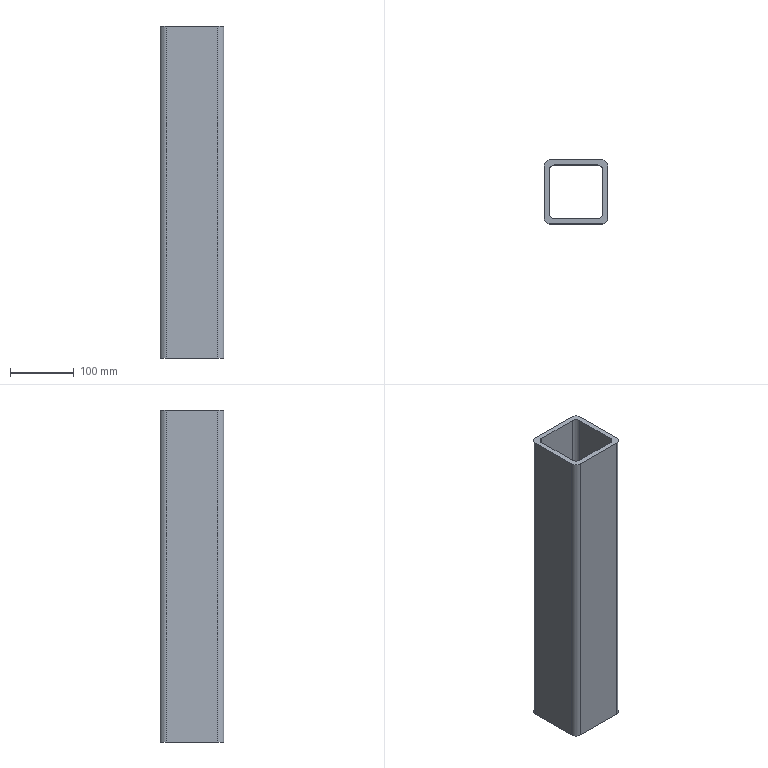Part | SolidWorks | features BaseBody 1 | 1 solid | 18 faces | box 100 x 100 x 520 mm | volume 1514811 mm3 | plane 10 | cylinder 8 | commonest cylinder face diameters 16 x4 20 x4
STEP:
#1=CARTESIAN_POINT('',(90.,-3.65,520.));
#2=VERTEX_POINT('',#1);
#3=CARTESIAN_POINT('',(90.,-3.65,0.));
#4=VERTEX_POINT('',#3);
#5=CARTESIAN_POINT('',(90.,-3.65,520.));
#6=DIRECTION('',(0.,0.,-1.));
#7=VECTOR('',#6,1000.);
#8=LINE('',#5,#7);
#9=EDGE_CURVE('',#2,#4,#8,.T.);
#10=ORIENTED_EDGE('',*,*,#9,.F.);
#11=CARTESIAN_POINT('',(10.,-3.65,520.));
#12=VERTEX_POINT('',#11);
#13=CARTESIAN_POINT('',(10.,-3.65,520.));
#14=DIRECTION('',(1.,0.,0.));
#15=VECTOR('',#14,1000.);
#16=LINE('',#13,#15);
#17=EDGE_CURVE('',#12,#2,#16,.T.);
#18=ORIENTED_EDGE('',*,*,#17,.F.);
#19=CARTESIAN_POINT('',(10.,-3.65,0.));
#20=VERTEX_POINT('',#19);
#21=CARTESIAN_POINT('',(10.,-3.65,520.));
#22=DIRECTION('',(0.,0.,1.));
#23=VECTOR('',#22,1000.);
#24=LINE('',#21,#23);
#25=EDGE_CURVE('',#20,#12,#24,.T.);
#26=ORIENTED_EDGE('',*,*,#25,.F.);
#27=CARTESIAN_POINT('',(10.,-3.65,0.));
#28=DIRECTION('',(-1.,0.,0.));
#29=VECTOR('',#28,1000.);
#30=LINE('',#27,#29);
#31=EDGE_CURVE('',#4,#20,#30,.T.);
#32=ORIENTED_EDGE('',*,*,#31,.F.);
#33=EDGE_LOOP('',(#10,#18,#26,#32));
#34=FACE_OUTER_BOUND('',#33,.T.);
#35=CARTESIAN_POINT('',(10.,-3.65,520.));
#36=DIRECTION('',(0.,1.,0.));
#37=DIRECTION('',(-1.,0.,0.));
#38=AXIS2_PLACEMENT_3D('',#35,#36,#37);
#39=PLANE('',#38);
#40=ADVANCED_FACE('',(#34),#39,.F.);
#41=CARTESIAN_POINT('',(84.,4.35,0.));
#42=VERTEX_POINT('',#41);
#43=CARTESIAN_POINT('',(16.,4.35,0.));
#44=VERTEX_POINT('',#43);
#45=CARTESIAN_POINT('',(10.,4.35,0.));
#46=DIRECTION('',(-1.,0.,0.));
#47=VECTOR('',#46,1000.);
#48=LINE('',#45,#47);
#49=EDGE_CURVE('',#42,#44,#48,.T.);
#50=ORIENTED_EDGE('',*,*,#49,.F.);
#51=CARTESIAN_POINT('',(92.,12.35,0.));
#52=VERTEX_POINT('',#51);
#53=CARTESIAN_POINT('',(84.,12.35,0.));
#54=DIRECTION('',(0.,0.,-1.));
#55=DIRECTION('',(-1.,0.,0.));
#56=AXIS2_PLACEMENT_3D('',#53,#54,#55);
#57=CIRCLE('',#56,8.);
#58=EDGE_CURVE('',#52,#42,#57,.T.);
#59=ORIENTED_EDGE('',*,*,#58,.F.);
#60=CARTESIAN_POINT('',(92.,80.35,0.));
#61=VERTEX_POINT('',#60);
#62=CARTESIAN_POINT('',(92.,6.35,0.));
#63=DIRECTION('',(0.,-1.,0.));
#64=VECTOR('',#63,1000.);
#65=LINE('',#62,#64);
#66=EDGE_CURVE('',#61,#52,#65,.T.);
#67=ORIENTED_EDGE('',*,*,#66,.F.);
#68=CARTESIAN_POINT('',(84.,88.35,0.));
#69=VERTEX_POINT('',#68);
#70=CARTESIAN_POINT('',(84.,80.35,0.));
#71=DIRECTION('',(0.,0.,-1.));
#72=DIRECTION('',(-1.,0.,0.));
#73=AXIS2_PLACEMENT_3D('',#70,#71,#72);
#74=CIRCLE('',#73,8.);
#75=EDGE_CURVE('',#69,#61,#74,.T.);
#76=ORIENTED_EDGE('',*,*,#75,.F.);
#77=CARTESIAN_POINT('',(16.,88.35,0.));
#78=VERTEX_POINT('',#77);
#79=CARTESIAN_POINT('',(10.,88.35,0.));
#80=DIRECTION('',(1.,0.,0.));
#81=VECTOR('',#80,1000.);
#82=LINE('',#79,#81);
#83=EDGE_CURVE('',#78,#69,#82,.T.);
#84=ORIENTED_EDGE('',*,*,#83,.F.);
#85=CARTESIAN_POINT('',(8.,80.35,0.));
#86=VERTEX_POINT('',#85);
#87=CARTESIAN_POINT('',(16.,80.35,0.));
#88=DIRECTION('',(0.,0.,-1.));
#89=DIRECTION('',(-1.,0.,0.));
#90=AXIS2_PLACEMENT_3D('',#87,#88,#89);
#91=CIRCLE('',#90,8.);
#92=EDGE_CURVE('',#86,#78,#91,.T.);
#93=ORIENTED_EDGE('',*,*,#92,.F.);
#94=CARTESIAN_POINT('',(8.,12.35,0.));
#95=VERTEX_POINT('',#94);
#96=CARTESIAN_POINT('',(8.,6.35,0.));
#97=DIRECTION('',(0.,1.,0.));
#98=VECTOR('',#97,1000.);
#99=LINE('',#96,#98);
#100=EDGE_CURVE('',#95,#86,#99,.T.);
#101=ORIENTED_EDGE('',*,*,#100,.F.);
#102=CARTESIAN_POINT('',(16.,12.35,0.));
#103=DIRECTION('',(0.,0.,-1.));
#104=DIRECTION('',(-1.,0.,0.));
#105=AXIS2_PLACEMENT_3D('',#102,#103,#104);
#106=CIRCLE('',#105,8.);
#107=EDGE_CURVE('',#44,#95,#106,.T.);
#108=ORIENTED_EDGE('',*,*,#107,.F.);
#109=EDGE_LOOP('',(#50,#59,#67,#76,#84,#93,#101,#108));
#110=FACE_BOUND('',#109,.T.);
#111=CARTESIAN_POINT('',(0.,86.35,0.));
#112=VERTEX_POINT('',#111);
#113=CARTESIAN_POINT('',(0.,6.35,0.));
#114=VERTEX_POINT('',#113);
#115=CARTESIAN_POINT('',(0.,6.35,0.));
#116=DIRECTION('',(0.,-1.,0.));
#117=VECTOR('',#116,1000.);
#118=LINE('',#115,#117);
#119=EDGE_CURVE('',#112,#114,#118,.T.);
#120=ORIENTED_EDGE('',*,*,#119,.F.);
#121=CARTESIAN_POINT('',(10.,96.35,0.));
#122=VERTEX_POINT('',#121);
#123=CARTESIAN_POINT('',(10.,86.35,0.));
#124=DIRECTION('',(0.,0.,1.));
#125=DIRECTION('',(-1.,0.,0.));
#126=AXIS2_PLACEMENT_3D('',#123,#124,#125);
#127=CIRCLE('',#126,10.);
#128=EDGE_CURVE('',#122,#112,#127,.T.);
#129=ORIENTED_EDGE('',*,*,#128,.F.);
#130=CARTESIAN_POINT('',(90.,96.35,0.));
#131=VERTEX_POINT('',#130);
#132=CARTESIAN_POINT('',(10.,96.35,0.));
#133=DIRECTION('',(-1.,0.,0.));
#134=VECTOR('',#133,1000.);
#135=LINE('',#132,#134);
#136=EDGE_CURVE('',#131,#122,#135,.T.);
#137=ORIENTED_EDGE('',*,*,#136,.F.);
#138=CARTESIAN_POINT('',(100.,86.35,0.));
#139=VERTEX_POINT('',#138);
#140=CARTESIAN_POINT('',(90.,86.35,0.));
#141=DIRECTION('',(0.,0.,1.));
#142=DIRECTION('',(-1.,0.,0.));
#143=AXIS2_PLACEMENT_3D('',#140,#141,#142);
#144=CIRCLE('',#143,10.);
#145=EDGE_CURVE('',#139,#131,#144,.T.);
#146=ORIENTED_EDGE('',*,*,#145,.F.);
#147=CARTESIAN_POINT('',(100.,6.35,0.));
#148=VERTEX_POINT('',#147);
#149=CARTESIAN_POINT('',(100.,6.35,0.));
#150=DIRECTION('',(0.,1.,0.));
#151=VECTOR('',#150,1000.);
#152=LINE('',#149,#151);
#153=EDGE_CURVE('',#148,#139,#152,.T.);
#154=ORIENTED_EDGE('',*,*,#153,.F.);
#155=CARTESIAN_POINT('',(90.,6.35,0.));
#156=DIRECTION('',(0.,0.,1.));
#157=DIRECTION('',(-1.,0.,0.));
#158=AXIS2_PLACEMENT_3D('',#155,#156,#157);
#159=CIRCLE('',#158,10.);
#160=EDGE_CURVE('',#4,#148,#159,.T.);
#161=ORIENTED_EDGE('',*,*,#160,.F.);
#162=ORIENTED_EDGE('',*,*,#31,.T.);
#163=CARTESIAN_POINT('',(10.,6.35,0.));
#164=DIRECTION('',(0.,0.,1.));
#165=DIRECTION('',(-1.,0.,0.));
#166=AXIS2_PLACEMENT_3D('',#163,#164,#165);
#167=CIRCLE('',#166,10.);
#168=EDGE_CURVE('',#114,#20,#167,.T.);
#169=ORIENTED_EDGE('',*,*,#168,.F.);
#170=EDGE_LOOP('',(#120,#129,#137,#146,#154,#161,#162,#169));
#171=FACE_OUTER_BOUND('',#170,.T.);
#172=CARTESIAN_POINT('',(10.,6.35,0.));
#173=DIRECTION('',(0.,0.,1.));
#174=DIRECTION('',(1.,0.,0.));
#175=AXIS2_PLACEMENT_3D('',#172,#173,#174);
#176=PLANE('',#175);
#177=ADVANCED_FACE('',(#110,#171),#176,.F.);
#178=CARTESIAN_POINT('',(100.,6.35,520.));
#179=VERTEX_POINT('',#178);
#180=CARTESIAN_POINT('',(90.,6.35,520.));
#181=DIRECTION('',(0.,0.,-1.));
#182=DIRECTION('',(-1.,0.,0.));
#183=AXIS2_PLACEMENT_3D('',#180,#181,#182);
#184=CIRCLE('',#183,10.);
#185=EDGE_CURVE('',#179,#2,#184,.T.);
#186=ORIENTED_EDGE('',*,*,#185,.T.);
#187=ORIENTED_EDGE('',*,*,#9,.T.);
#188=ORIENTED_EDGE('',*,*,#160,.T.);
#189=CARTESIAN_POINT('',(100.,6.35,520.));
#190=DIRECTION('',(0.,0.,1.));
#191=VECTOR('',#190,1000.);
#192=LINE('',#189,#191);
#193=EDGE_CURVE('',#148,#179,#192,.T.);
#194=ORIENTED_EDGE('',*,*,#193,.T.);
#195=EDGE_LOOP('',(#186,#187,#188,#194));
#196=FACE_OUTER_BOUND('',#195,.T.);
#197=CARTESIAN_POINT('',(90.,6.35,520.));
#198=DIRECTION('',(0.,0.,-1.));
#199=DIRECTION('',(-1.,0.,0.));
#200=AXIS2_PLACEMENT_3D('',#197,#198,#199);
#201=CYLINDRICAL_SURFACE('',#200,10.);
#202=ADVANCED_FACE('',(#196),#201,.T.);
#203=CARTESIAN_POINT('',(92.,80.35,520.));
#204=VERTEX_POINT('',#203);
#205=CARTESIAN_POINT('',(92.,12.35,520.));
#206=VERTEX_POINT('',#205);
#207=CARTESIAN_POINT('',(92.,6.35,520.));
#208=DIRECTION('',(0.,-1.,0.));
#209=VECTOR('',#208,1000.);
#210=LINE('',#207,#209);
#211=EDGE_CURVE('',#204,#206,#210,.T.);
#212=ORIENTED_EDGE('',*,*,#211,.T.);
#213=CARTESIAN_POINT('',(84.,4.35,520.));
#214=VERTEX_POINT('',#213);
#215=CARTESIAN_POINT('',(84.,12.35,520.));
#216=DIRECTION('',(0.,0.,-1.));
#217=DIRECTION('',(-1.,0.,0.));
#218=AXIS2_PLACEMENT_3D('',#215,#216,#217);
#219=CIRCLE('',#218,8.);
#220=EDGE_CURVE('',#206,#214,#219,.T.);
#221=ORIENTED_EDGE('',*,*,#220,.T.);
#222=CARTESIAN_POINT('',(16.,4.35,520.));
#223=VERTEX_POINT('',#222);
#224=CARTESIAN_POINT('',(10.,4.35,520.));
#225=DIRECTION('',(-1.,0.,0.));
#226=VECTOR('',#225,1000.);
#227=LINE('',#224,#226);
#228=EDGE_CURVE('',#214,#223,#227,.T.);
#229=ORIENTED_EDGE('',*,*,#228,.T.);
#230=CARTESIAN_POINT('',(8.,12.35,520.));
#231=VERTEX_POINT('',#230);
#232=CARTESIAN_POINT('',(16.,12.35,520.));
#233=DIRECTION('',(0.,0.,-1.));
#234=DIRECTION('',(-1.,0.,0.));
#235=AXIS2_PLACEMENT_3D('',#232,#233,#234);
#236=CIRCLE('',#235,8.);
#237=EDGE_CURVE('',#223,#231,#236,.T.);
#238=ORIENTED_EDGE('',*,*,#237,.T.);
#239=CARTESIAN_POINT('',(8.,80.35,520.));
#240=VERTEX_POINT('',#239);
#241=CARTESIAN_POINT('',(8.,6.35,520.));
#242=DIRECTION('',(0.,1.,0.));
#243=VECTOR('',#242,1000.);
#244=LINE('',#241,#243);
#245=EDGE_CURVE('',#231,#240,#244,.T.);
#246=ORIENTED_EDGE('',*,*,#245,.T.);
#247=CARTESIAN_POINT('',(16.,88.35,520.));
#248=VERTEX_POINT('',#247);
#249=CARTESIAN_POINT('',(16.,80.35,520.));
#250=DIRECTION('',(0.,0.,-1.));
#251=DIRECTION('',(-1.,0.,0.));
#252=AXIS2_PLACEMENT_3D('',#249,#250,#251);
#253=CIRCLE('',#252,8.);
#254=EDGE_CURVE('',#240,#248,#253,.T.);
#255=ORIENTED_EDGE('',*,*,#254,.T.);
#256=CARTESIAN_POINT('',(84.,88.35,520.));
#257=VERTEX_POINT('',#256);
#258=CARTESIAN_POINT('',(10.,88.35,520.));
#259=DIRECTION('',(1.,0.,0.));
#260=VECTOR('',#259,1000.);
#261=LINE('',#258,#260);
#262=EDGE_CURVE('',#248,#257,#261,.T.);
#263=ORIENTED_EDGE('',*,*,#262,.T.);
#264=CARTESIAN_POINT('',(84.,80.35,520.));
#265=DIRECTION('',(0.,0.,-1.));
#266=DIRECTION('',(-1.,0.,0.));
#267=AXIS2_PLACEMENT_3D('',#264,#265,#266);
#268=CIRCLE('',#267,8.);
#269=EDGE_CURVE('',#257,#204,#268,.T.);
#270=ORIENTED_EDGE('',*,*,#269,.T.);
#271=EDGE_LOOP('',(#212,#221,#229,#238,#246,#255,#263,#270));
#272=FACE_BOUND('',#271,.T.);
#273=CARTESIAN_POINT('',(10.,96.35,520.));
#274=VERTEX_POINT('',#273);
#275=CARTESIAN_POINT('',(0.,86.35,520.));
#276=VERTEX_POINT('',#275);
#277=CARTESIAN_POINT('',(10.,86.35,520.));
#278=DIRECTION('',(0.,0.,1.));
#279=DIRECTION('',(-1.,0.,0.));
#280=AXIS2_PLACEMENT_3D('',#277,#278,#279);
#281=CIRCLE('',#280,10.);
#282=EDGE_CURVE('',#274,#276,#281,.T.);
#283=ORIENTED_EDGE('',*,*,#282,.T.);
#284=CARTESIAN_POINT('',(0.,6.35,520.));
#285=VERTEX_POINT('',#284);
#286=CARTESIAN_POINT('',(0.,6.35,520.));
#287=DIRECTION('',(0.,-1.,0.));
#288=VECTOR('',#287,1000.);
#289=LINE('',#286,#288);
#290=EDGE_CURVE('',#276,#285,#289,.T.);
#291=ORIENTED_EDGE('',*,*,#290,.T.);
#292=CARTESIAN_POINT('',(10.,6.35,520.));
#293=DIRECTION('',(0.,0.,1.));
#294=DIRECTION('',(-1.,0.,0.));
#295=AXIS2_PLACEMENT_3D('',#292,#293,#294);
#296=CIRCLE('',#295,10.);
#297=EDGE_CURVE('',#285,#12,#296,.T.);
#298=ORIENTED_EDGE('',*,*,#297,.T.);
#299=ORIENTED_EDGE('',*,*,#17,.T.);
#300=ORIENTED_EDGE('',*,*,#185,.F.);
#301=CARTESIAN_POINT('',(100.,86.35,520.));
#302=VERTEX_POINT('',#301);
#303=CARTESIAN_POINT('',(100.,6.35,520.));
#304=DIRECTION('',(0.,1.,0.));
#305=VECTOR('',#304,1000.);
#306=LINE('',#303,#305);
#307=EDGE_CURVE('',#179,#302,#306,.T.);
#308=ORIENTED_EDGE('',*,*,#307,.T.);
#309=CARTESIAN_POINT('',(90.,96.35,520.));
#310=VERTEX_POINT('',#309);
#311=CARTESIAN_POINT('',(90.,86.35,520.));
#312=DIRECTION('',(0.,0.,1.));
#313=DIRECTION('',(-1.,0.,0.));
#314=AXIS2_PLACEMENT_3D('',#311,#312,#313);
#315=CIRCLE('',#314,10.);
#316=EDGE_CURVE('',#302,#310,#315,.T.);
#317=ORIENTED_EDGE('',*,*,#316,.T.);
#318=CARTESIAN_POINT('',(10.,96.35,520.));
#319=DIRECTION('',(-1.,0.,0.));
#320=VECTOR('',#319,1000.);
#321=LINE('',#318,#320);
#322=EDGE_CURVE('',#310,#274,#321,.T.);
#323=ORIENTED_EDGE('',*,*,#322,.T.);
#324=EDGE_LOOP('',(#283,#291,#298,#299,#300,#308,#317,#323));
#325=FACE_OUTER_BOUND('',#324,.T.);
#326=CARTESIAN_POINT('',(10.,6.35,520.));
#327=DIRECTION('',(0.,0.,1.));
#328=DIRECTION('',(1.,0.,0.));
#329=AXIS2_PLACEMENT_3D('',#326,#327,#328);
#330=PLANE('',#329);
#331=ADVANCED_FACE('',(#272,#325),#330,.T.);
#332=ORIENTED_EDGE('',*,*,#297,.F.);
#333=CARTESIAN_POINT('',(0.,6.35,520.));
#334=DIRECTION('',(0.,0.,-1.));
#335=VECTOR('',#334,1000.);
#336=LINE('',#333,#335);
#337=EDGE_CURVE('',#285,#114,#336,.T.);
#338=ORIENTED_EDGE('',*,*,#337,.T.);
#339=ORIENTED_EDGE('',*,*,#168,.T.);
#340=ORIENTED_EDGE('',*,*,#25,.T.);
#341=EDGE_LOOP('',(#332,#338,#339,#340));
#342=FACE_OUTER_BOUND('',#341,.T.);
#343=CARTESIAN_POINT('',(10.,6.35,520.));
#344=DIRECTION('',(0.,0.,-1.));
#345=DIRECTION('',(-1.,0.,0.));
#346=AXIS2_PLACEMENT_3D('',#343,#344,#345);
#347=CYLINDRICAL_SURFACE('',#346,10.);
#348=ADVANCED_FACE('',(#342),#347,.T.);
#349=CARTESIAN_POINT('',(8.,12.35,520.));
#350=DIRECTION('',(0.,0.,-1.));
#351=VECTOR('',#350,1000.);
#352=LINE('',#349,#351);
#353=EDGE_CURVE('',#231,#95,#352,.T.);
#354=ORIENTED_EDGE('',*,*,#353,.F.);
#355=ORIENTED_EDGE('',*,*,#237,.F.);
#356=CARTESIAN_POINT('',(16.,4.35,520.));
#357=DIRECTION('',(0.,0.,1.));
#358=VECTOR('',#357,1000.);
#359=LINE('',#356,#358);
#360=EDGE_CURVE('',#44,#223,#359,.T.);
#361=ORIENTED_EDGE('',*,*,#360,.F.);
#362=ORIENTED_EDGE('',*,*,#107,.T.);
#363=EDGE_LOOP('',(#354,#355,#361,#362));
#364=FACE_OUTER_BOUND('',#363,.T.);
#365=CARTESIAN_POINT('',(16.,12.35,520.));
#366=DIRECTION('',(0.,0.,-1.));
#367=DIRECTION('',(-1.,0.,0.));
#368=AXIS2_PLACEMENT_3D('',#365,#366,#367);
#369=CYLINDRICAL_SURFACE('',#368,8.);
#370=ADVANCED_FACE('',(#364),#369,.F.);
#371=ORIENTED_EDGE('',*,*,#228,.F.);
#372=CARTESIAN_POINT('',(84.,4.35,520.));
#373=DIRECTION('',(0.,0.,-1.));
#374=VECTOR('',#373,1000.);
#375=LINE('',#372,#374);
#376=EDGE_CURVE('',#214,#42,#375,.T.);
#377=ORIENTED_EDGE('',*,*,#376,.T.);
#378=ORIENTED_EDGE('',*,*,#49,.T.);
#379=ORIENTED_EDGE('',*,*,#360,.T.);
#380=EDGE_LOOP('',(#371,#377,#378,#379));
#381=FACE_OUTER_BOUND('',#380,.T.);
#382=CARTESIAN_POINT('',(16.,4.35,520.));
#383=DIRECTION('',(0.,1.,0.));
#384=DIRECTION('',(-1.,0.,0.));
#385=AXIS2_PLACEMENT_3D('',#382,#383,#384);
#386=PLANE('',#385);
#387=ADVANCED_FACE('',(#381),#386,.T.);
#388=ORIENTED_EDGE('',*,*,#376,.F.);
#389=ORIENTED_EDGE('',*,*,#220,.F.);
#390=CARTESIAN_POINT('',(92.,12.35,520.));
#391=DIRECTION('',(0.,0.,1.));
#392=VECTOR('',#391,1000.);
#393=LINE('',#390,#392);
#394=EDGE_CURVE('',#52,#206,#393,.T.);
#395=ORIENTED_EDGE('',*,*,#394,.F.);
#396=ORIENTED_EDGE('',*,*,#58,.T.);
#397=EDGE_LOOP('',(#388,#389,#395,#396));
#398=FACE_OUTER_BOUND('',#397,.T.);
#399=CARTESIAN_POINT('',(84.,12.35,520.));
#400=DIRECTION('',(0.,0.,-1.));
#401=DIRECTION('',(-1.,0.,0.));
#402=AXIS2_PLACEMENT_3D('',#399,#400,#401);
#403=CYLINDRICAL_SURFACE('',#402,8.);
#404=ADVANCED_FACE('',(#398),#403,.F.);
#405=ORIENTED_EDGE('',*,*,#394,.T.);
#406=ORIENTED_EDGE('',*,*,#211,.F.);
#407=CARTESIAN_POINT('',(92.,80.35,520.));
#408=DIRECTION('',(0.,0.,1.));
#409=VECTOR('',#408,1000.);
#410=LINE('',#407,#409);
#411=EDGE_CURVE('',#61,#204,#410,.T.);
#412=ORIENTED_EDGE('',*,*,#411,.F.);
#413=ORIENTED_EDGE('',*,*,#66,.T.);
#414=EDGE_LOOP('',(#405,#406,#412,#413));
#415=FACE_OUTER_BOUND('',#414,.T.);
#416=CARTESIAN_POINT('',(92.,80.35,520.));
#417=DIRECTION('',(1.,0.,0.));
#418=DIRECTION('',(0.,1.,0.));
#419=AXIS2_PLACEMENT_3D('',#416,#417,#418);
#420=PLANE('',#419);
#421=ADVANCED_FACE('',(#415),#420,.F.);
#422=ORIENTED_EDGE('',*,*,#411,.T.);
#423=ORIENTED_EDGE('',*,*,#269,.F.);
#424=CARTESIAN_POINT('',(84.,88.35,520.));
#425=DIRECTION('',(0.,0.,1.));
#426=VECTOR('',#425,1000.);
#427=LINE('',#424,#426);
#428=EDGE_CURVE('',#69,#257,#427,.T.);
#429=ORIENTED_EDGE('',*,*,#428,.F.);
#430=ORIENTED_EDGE('',*,*,#75,.T.);
#431=EDGE_LOOP('',(#422,#423,#429,#430));
#432=FACE_OUTER_BOUND('',#431,.T.);
#433=CARTESIAN_POINT('',(84.,80.35,520.));
#434=DIRECTION('',(0.,0.,-1.));
#435=DIRECTION('',(-1.,0.,0.));
#436=AXIS2_PLACEMENT_3D('',#433,#434,#435);
#437=CYLINDRICAL_SURFACE('',#436,8.);
#438=ADVANCED_FACE('',(#432),#437,.F.);
#439=ORIENTED_EDGE('',*,*,#262,.F.);
#440=CARTESIAN_POINT('',(16.,88.35,520.));
#441=DIRECTION('',(0.,0.,-1.));
#442=VECTOR('',#441,1000.);
#443=LINE('',#440,#442);
#444=EDGE_CURVE('',#248,#78,#443,.T.);
#445=ORIENTED_EDGE('',*,*,#444,.T.);
#446=ORIENTED_EDGE('',*,*,#83,.T.);
#447=ORIENTED_EDGE('',*,*,#428,.T.);
#448=EDGE_LOOP('',(#439,#445,#446,#447));
#449=FACE_OUTER_BOUND('',#448,.T.);
#450=CARTESIAN_POINT('',(84.,88.35,520.));
#451=DIRECTION('',(0.,-1.,0.));
#452=DIRECTION('',(1.,0.,0.));
#453=AXIS2_PLACEMENT_3D('',#450,#451,#452);
#454=PLANE('',#453);
#455=ADVANCED_FACE('',(#449),#454,.T.);
#456=ORIENTED_EDGE('',*,*,#444,.F.);
#457=ORIENTED_EDGE('',*,*,#254,.F.);
#458=CARTESIAN_POINT('',(8.,80.35,520.));
#459=DIRECTION('',(0.,0.,1.));
#460=VECTOR('',#459,1000.);
#461=LINE('',#458,#460);
#462=EDGE_CURVE('',#86,#240,#461,.T.);
#463=ORIENTED_EDGE('',*,*,#462,.F.);
#464=ORIENTED_EDGE('',*,*,#92,.T.);
#465=EDGE_LOOP('',(#456,#457,#463,#464));
#466=FACE_OUTER_BOUND('',#465,.T.);
#467=CARTESIAN_POINT('',(16.,80.35,520.));
#468=DIRECTION('',(0.,0.,-1.));
#469=DIRECTION('',(-1.,0.,0.));
#470=AXIS2_PLACEMENT_3D('',#467,#468,#469);
#471=CYLINDRICAL_SURFACE('',#470,8.);
#472=ADVANCED_FACE('',(#466),#471,.F.);
#473=ORIENTED_EDGE('',*,*,#462,.T.);
#474=ORIENTED_EDGE('',*,*,#245,.F.);
#475=ORIENTED_EDGE('',*,*,#353,.T.);
#476=ORIENTED_EDGE('',*,*,#100,.T.);
#477=EDGE_LOOP('',(#473,#474,#475,#476));
#478=FACE_OUTER_BOUND('',#477,.T.);
#479=CARTESIAN_POINT('',(8.,12.35,520.));
#480=DIRECTION('',(-1.,0.,0.));
#481=DIRECTION('',(0.,-1.,0.));
#482=AXIS2_PLACEMENT_3D('',#479,#480,#481);
#483=PLANE('',#482);
#484=ADVANCED_FACE('',(#478),#483,.F.);
#485=ORIENTED_EDGE('',*,*,#290,.F.);
#486=CARTESIAN_POINT('',(0.,86.35,520.));
#487=DIRECTION('',(0.,0.,-1.));
#488=VECTOR('',#487,1000.);
#489=LINE('',#486,#488);
#490=EDGE_CURVE('',#276,#112,#489,.T.);
#491=ORIENTED_EDGE('',*,*,#490,.T.);
#492=ORIENTED_EDGE('',*,*,#119,.T.);
#493=ORIENTED_EDGE('',*,*,#337,.F.);
#494=EDGE_LOOP('',(#485,#491,#492,#493));
#495=FACE_OUTER_BOUND('',#494,.T.);
#496=CARTESIAN_POINT('',(0.,6.35,520.));
#497=DIRECTION('',(-1.,0.,0.));
#498=DIRECTION('',(0.,-1.,0.));
#499=AXIS2_PLACEMENT_3D('',#496,#497,#498);
#500=PLANE('',#499);
#501=ADVANCED_FACE('',(#495),#500,.T.);
#502=ORIENTED_EDGE('',*,*,#282,.F.);
#503=CARTESIAN_POINT('',(10.,96.35,520.));
#504=DIRECTION('',(0.,0.,-1.));
#505=VECTOR('',#504,1000.);
#506=LINE('',#503,#505);
#507=EDGE_CURVE('',#274,#122,#506,.T.);
#508=ORIENTED_EDGE('',*,*,#507,.T.);
#509=ORIENTED_EDGE('',*,*,#128,.T.);
#510=ORIENTED_EDGE('',*,*,#490,.F.);
#511=EDGE_LOOP('',(#502,#508,#509,#510));
#512=FACE_OUTER_BOUND('',#511,.T.);
#513=CARTESIAN_POINT('',(10.,86.35,520.));
#514=DIRECTION('',(0.,0.,-1.));
#515=DIRECTION('',(-1.,0.,0.));
#516=AXIS2_PLACEMENT_3D('',#513,#514,#515);
#517=CYLINDRICAL_SURFACE('',#516,10.);
#518=ADVANCED_FACE('',(#512),#517,.T.);
#519=ORIENTED_EDGE('',*,*,#507,.F.);
#520=ORIENTED_EDGE('',*,*,#322,.F.);
#521=CARTESIAN_POINT('',(90.,96.35,520.));
#522=DIRECTION('',(0.,0.,1.));
#523=VECTOR('',#522,1000.);
#524=LINE('',#521,#523);
#525=EDGE_CURVE('',#131,#310,#524,.T.);
#526=ORIENTED_EDGE('',*,*,#525,.F.);
#527=ORIENTED_EDGE('',*,*,#136,.T.);
#528=EDGE_LOOP('',(#519,#520,#526,#527));
#529=FACE_OUTER_BOUND('',#528,.T.);
#530=CARTESIAN_POINT('',(90.,96.35,520.));
#531=DIRECTION('',(0.,-1.,0.));
#532=DIRECTION('',(1.,0.,0.));
#533=AXIS2_PLACEMENT_3D('',#530,#531,#532);
#534=PLANE('',#533);
#535=ADVANCED_FACE('',(#529),#534,.F.);
#536=ORIENTED_EDGE('',*,*,#316,.F.);
#537=CARTESIAN_POINT('',(100.,86.35,520.));
#538=DIRECTION('',(0.,0.,-1.));
#539=VECTOR('',#538,1000.);
#540=LINE('',#537,#539);
#541=EDGE_CURVE('',#302,#139,#540,.T.);
#542=ORIENTED_EDGE('',*,*,#541,.T.);
#543=ORIENTED_EDGE('',*,*,#145,.T.);
#544=ORIENTED_EDGE('',*,*,#525,.T.);
#545=EDGE_LOOP('',(#536,#542,#543,#544));
#546=FACE_OUTER_BOUND('',#545,.T.);
#547=CARTESIAN_POINT('',(90.,86.35,520.));
#548=DIRECTION('',(0.,0.,-1.));
#549=DIRECTION('',(-1.,0.,0.));
#550=AXIS2_PLACEMENT_3D('',#547,#548,#549);
#551=CYLINDRICAL_SURFACE('',#550,10.);
#552=ADVANCED_FACE('',(#546),#551,.T.);
#553=ORIENTED_EDGE('',*,*,#307,.F.);
#554=ORIENTED_EDGE('',*,*,#193,.F.);
#555=ORIENTED_EDGE('',*,*,#153,.T.);
#556=ORIENTED_EDGE('',*,*,#541,.F.);
#557=EDGE_LOOP('',(#553,#554,#555,#556));
#558=FACE_OUTER_BOUND('',#557,.T.);
#559=CARTESIAN_POINT('',(100.,86.35,520.));
#560=DIRECTION('',(1.,0.,0.));
#561=DIRECTION('',(0.,0.,-1.));
#562=AXIS2_PLACEMENT_3D('',#559,#560,#561);
#563=PLANE('',#562);
#564=ADVANCED_FACE('',(#558),#563,.T.);
#565=CLOSED_SHELL('',(#40,#177,#202,#331,#348,#370,#387,#404,#421,#438,#455,#472,#484,#501,#518,#535,#552,#564));
#566=MANIFOLD_SOLID_BREP('',#565);
#567=CARTESIAN_POINT('',(0.,0.,0.));
#568=DIRECTION('',(0.,0.,1.));
#569=DIRECTION('',(1.,0.,0.));
#570=AXIS2_PLACEMENT_3D('',#567,#568,#569);
#571=(LENGTH_UNIT()NAMED_UNIT(*)SI_UNIT(.MILLI.,.METRE.));
#572=UNCERTAINTY_MEASURE_WITH_UNIT(LENGTH_MEASURE(0.00001),#571,'','');
#573=(NAMED_UNIT(*)PLANE_ANGLE_UNIT()SI_UNIT($,.RADIAN.));
#574=(NAMED_UNIT(*)SI_UNIT($,.STERADIAN.)SOLID_ANGLE_UNIT());
#575=(GEOMETRIC_REPRESENTATION_CONTEXT(3)GLOBAL_UNCERTAINTY_ASSIGNED_CONTEXT((#572))GLOBAL_UNIT_ASSIGNED_CONTEXT((#571,#573,#574))REPRESENTATION_CONTEXT('',''));
#576=ADVANCED_BREP_SHAPE_REPRESENTATION('',(#566,#570),#575);